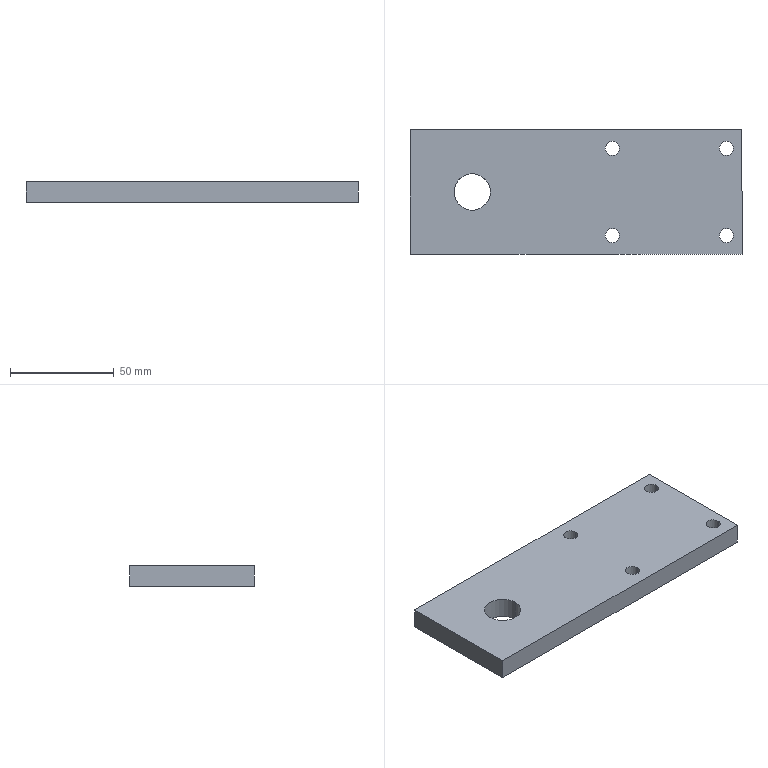Part | SolidWorks | features HoleWzd 2, Extrusion 1 | 1 solid | 16 faces | box 160 x 60 x 10 mm | volume 92142 mm3 | cylinder 10 | plane 6 | commonest cylinder face diameters 6.8 x8 17.5 x2
STEP:
#1=CARTESIAN_POINT('',(14.1,21.,0.));
#2=VERTEX_POINT('',#1);
#3=CARTESIAN_POINT('',(20.9,21.,0.));
#4=VERTEX_POINT('',#3);
#5=CARTESIAN_POINT('',(17.5,21.,0.));
#6=DIRECTION('',(0.,0.,1.));
#7=DIRECTION('',(1.,0.,0.));
#8=AXIS2_PLACEMENT_3D('',#5,#6,#7);
#9=CIRCLE('',#8,3.4);
#10=EDGE_CURVE('',#2,#4,#9,.T.);
#11=ORIENTED_EDGE('',*,*,#10,.F.);
#12=CARTESIAN_POINT('',(14.1,21.,10.));
#13=VERTEX_POINT('',#12);
#14=CARTESIAN_POINT('',(14.1,21.,10.));
#15=DIRECTION('',(0.,0.,1.));
#16=VECTOR('',#15,1000.);
#17=LINE('',#14,#16);
#18=EDGE_CURVE('',#2,#13,#17,.T.);
#19=ORIENTED_EDGE('',*,*,#18,.T.);
#20=CARTESIAN_POINT('',(20.9,21.,10.));
#21=VERTEX_POINT('',#20);
#22=CARTESIAN_POINT('',(17.5,21.,10.));
#23=DIRECTION('',(0.,0.,1.));
#24=DIRECTION('',(1.,0.,0.));
#25=AXIS2_PLACEMENT_3D('',#22,#23,#24);
#26=CIRCLE('',#25,3.4);
#27=EDGE_CURVE('',#13,#21,#26,.T.);
#28=ORIENTED_EDGE('',*,*,#27,.T.);
#29=CARTESIAN_POINT('',(20.9,21.,10.));
#30=DIRECTION('',(0.,0.,1.));
#31=VECTOR('',#30,1000.);
#32=LINE('',#29,#31);
#33=EDGE_CURVE('',#4,#21,#32,.T.);
#34=ORIENTED_EDGE('',*,*,#33,.F.);
#35=EDGE_LOOP('',(#11,#19,#28,#34));
#36=FACE_OUTER_BOUND('',#35,.T.);
#37=CARTESIAN_POINT('',(17.5,21.,10.));
#38=DIRECTION('',(0.,0.,1.));
#39=DIRECTION('',(1.,0.,0.));
#40=AXIS2_PLACEMENT_3D('',#37,#38,#39);
#41=CYLINDRICAL_SURFACE('',#40,3.4);
#42=ADVANCED_FACE('',(#36),#41,.F.);
#43=CARTESIAN_POINT('',(69.1,21.,0.));
#44=VERTEX_POINT('',#43);
#45=CARTESIAN_POINT('',(75.9,21.,0.));
#46=VERTEX_POINT('',#45);
#47=CARTESIAN_POINT('',(72.5,21.,0.));
#48=DIRECTION('',(0.,0.,1.));
#49=DIRECTION('',(1.,0.,0.));
#50=AXIS2_PLACEMENT_3D('',#47,#48,#49);
#51=CIRCLE('',#50,3.4);
#52=EDGE_CURVE('',#44,#46,#51,.T.);
#53=ORIENTED_EDGE('',*,*,#52,.F.);
#54=CARTESIAN_POINT('',(69.1,21.,10.));
#55=VERTEX_POINT('',#54);
#56=CARTESIAN_POINT('',(69.1,21.,10.));
#57=DIRECTION('',(0.,0.,1.));
#58=VECTOR('',#57,1000.);
#59=LINE('',#56,#58);
#60=EDGE_CURVE('',#44,#55,#59,.T.);
#61=ORIENTED_EDGE('',*,*,#60,.T.);
#62=CARTESIAN_POINT('',(75.9,21.,10.));
#63=VERTEX_POINT('',#62);
#64=CARTESIAN_POINT('',(72.5,21.,10.));
#65=DIRECTION('',(0.,0.,1.));
#66=DIRECTION('',(1.,0.,0.));
#67=AXIS2_PLACEMENT_3D('',#64,#65,#66);
#68=CIRCLE('',#67,3.4);
#69=EDGE_CURVE('',#55,#63,#68,.T.);
#70=ORIENTED_EDGE('',*,*,#69,.T.);
#71=CARTESIAN_POINT('',(75.9,21.,10.));
#72=DIRECTION('',(0.,0.,1.));
#73=VECTOR('',#72,1000.);
#74=LINE('',#71,#73);
#75=EDGE_CURVE('',#46,#63,#74,.T.);
#76=ORIENTED_EDGE('',*,*,#75,.F.);
#77=EDGE_LOOP('',(#53,#61,#70,#76));
#78=FACE_OUTER_BOUND('',#77,.T.);
#79=CARTESIAN_POINT('',(72.5,21.,10.));
#80=DIRECTION('',(0.,0.,1.));
#81=DIRECTION('',(1.,0.,0.));
#82=AXIS2_PLACEMENT_3D('',#79,#80,#81);
#83=CYLINDRICAL_SURFACE('',#82,3.4);
#84=ADVANCED_FACE('',(#78),#83,.F.);
#85=CARTESIAN_POINT('',(14.1,-21.,0.));
#86=VERTEX_POINT('',#85);
#87=CARTESIAN_POINT('',(20.9,-21.,0.));
#88=VERTEX_POINT('',#87);
#89=CARTESIAN_POINT('',(17.5,-21.,0.));
#90=DIRECTION('',(0.,0.,1.));
#91=DIRECTION('',(1.,0.,0.));
#92=AXIS2_PLACEMENT_3D('',#89,#90,#91);
#93=CIRCLE('',#92,3.4);
#94=EDGE_CURVE('',#86,#88,#93,.T.);
#95=ORIENTED_EDGE('',*,*,#94,.F.);
#96=CARTESIAN_POINT('',(14.1,-21.,10.));
#97=VERTEX_POINT('',#96);
#98=CARTESIAN_POINT('',(14.1,-21.,10.));
#99=DIRECTION('',(0.,0.,1.));
#100=VECTOR('',#99,1000.);
#101=LINE('',#98,#100);
#102=EDGE_CURVE('',#86,#97,#101,.T.);
#103=ORIENTED_EDGE('',*,*,#102,.T.);
#104=CARTESIAN_POINT('',(20.9,-21.,10.));
#105=VERTEX_POINT('',#104);
#106=CARTESIAN_POINT('',(17.5,-21.,10.));
#107=DIRECTION('',(0.,0.,1.));
#108=DIRECTION('',(1.,0.,0.));
#109=AXIS2_PLACEMENT_3D('',#106,#107,#108);
#110=CIRCLE('',#109,3.4);
#111=EDGE_CURVE('',#97,#105,#110,.T.);
#112=ORIENTED_EDGE('',*,*,#111,.T.);
#113=CARTESIAN_POINT('',(20.9,-21.,10.));
#114=DIRECTION('',(0.,0.,1.));
#115=VECTOR('',#114,1000.);
#116=LINE('',#113,#115);
#117=EDGE_CURVE('',#88,#105,#116,.T.);
#118=ORIENTED_EDGE('',*,*,#117,.F.);
#119=EDGE_LOOP('',(#95,#103,#112,#118));
#120=FACE_OUTER_BOUND('',#119,.T.);
#121=CARTESIAN_POINT('',(17.5,-21.,10.));
#122=DIRECTION('',(0.,0.,1.));
#123=DIRECTION('',(1.,0.,0.));
#124=AXIS2_PLACEMENT_3D('',#121,#122,#123);
#125=CYLINDRICAL_SURFACE('',#124,3.4);
#126=ADVANCED_FACE('',(#120),#125,.F.);
#127=CARTESIAN_POINT('',(69.1,-21.,0.));
#128=VERTEX_POINT('',#127);
#129=CARTESIAN_POINT('',(75.9,-21.,0.));
#130=VERTEX_POINT('',#129);
#131=CARTESIAN_POINT('',(72.5,-21.,0.));
#132=DIRECTION('',(0.,0.,1.));
#133=DIRECTION('',(1.,0.,0.));
#134=AXIS2_PLACEMENT_3D('',#131,#132,#133);
#135=CIRCLE('',#134,3.4);
#136=EDGE_CURVE('',#128,#130,#135,.T.);
#137=ORIENTED_EDGE('',*,*,#136,.F.);
#138=CARTESIAN_POINT('',(69.1,-21.,10.));
#139=VERTEX_POINT('',#138);
#140=CARTESIAN_POINT('',(69.1,-21.,10.));
#141=DIRECTION('',(0.,0.,1.));
#142=VECTOR('',#141,1000.);
#143=LINE('',#140,#142);
#144=EDGE_CURVE('',#128,#139,#143,.T.);
#145=ORIENTED_EDGE('',*,*,#144,.T.);
#146=CARTESIAN_POINT('',(75.9,-21.,10.));
#147=VERTEX_POINT('',#146);
#148=CARTESIAN_POINT('',(72.5,-21.,10.));
#149=DIRECTION('',(0.,0.,1.));
#150=DIRECTION('',(1.,0.,0.));
#151=AXIS2_PLACEMENT_3D('',#148,#149,#150);
#152=CIRCLE('',#151,3.4);
#153=EDGE_CURVE('',#139,#147,#152,.T.);
#154=ORIENTED_EDGE('',*,*,#153,.T.);
#155=CARTESIAN_POINT('',(75.9,-21.,10.));
#156=DIRECTION('',(0.,0.,1.));
#157=VECTOR('',#156,1000.);
#158=LINE('',#155,#157);
#159=EDGE_CURVE('',#130,#147,#158,.T.);
#160=ORIENTED_EDGE('',*,*,#159,.F.);
#161=EDGE_LOOP('',(#137,#145,#154,#160));
#162=FACE_OUTER_BOUND('',#161,.T.);
#163=CARTESIAN_POINT('',(72.5,-21.,10.));
#164=DIRECTION('',(0.,0.,1.));
#165=DIRECTION('',(1.,0.,0.));
#166=AXIS2_PLACEMENT_3D('',#163,#164,#165);
#167=CYLINDRICAL_SURFACE('',#166,3.4);
#168=ADVANCED_FACE('',(#162),#167,.F.);
#169=CARTESIAN_POINT('',(-58.75,0.,0.));
#170=VERTEX_POINT('',#169);
#171=CARTESIAN_POINT('',(-41.25,0.,0.));
#172=VERTEX_POINT('',#171);
#173=CARTESIAN_POINT('',(-50.,0.,0.));
#174=DIRECTION('',(0.,0.,1.));
#175=DIRECTION('',(1.,0.,0.));
#176=AXIS2_PLACEMENT_3D('',#173,#174,#175);
#177=CIRCLE('',#176,8.75);
#178=EDGE_CURVE('',#170,#172,#177,.T.);
#179=ORIENTED_EDGE('',*,*,#178,.F.);
#180=CARTESIAN_POINT('',(-58.75,0.,10.));
#181=VERTEX_POINT('',#180);
#182=CARTESIAN_POINT('',(-58.75,0.,10.));
#183=DIRECTION('',(0.,0.,1.));
#184=VECTOR('',#183,1000.);
#185=LINE('',#182,#184);
#186=EDGE_CURVE('',#170,#181,#185,.T.);
#187=ORIENTED_EDGE('',*,*,#186,.T.);
#188=CARTESIAN_POINT('',(-41.25,0.,10.));
#189=VERTEX_POINT('',#188);
#190=CARTESIAN_POINT('',(-50.,0.,10.));
#191=DIRECTION('',(0.,0.,1.));
#192=DIRECTION('',(1.,0.,0.));
#193=AXIS2_PLACEMENT_3D('',#190,#191,#192);
#194=CIRCLE('',#193,8.75);
#195=EDGE_CURVE('',#181,#189,#194,.T.);
#196=ORIENTED_EDGE('',*,*,#195,.T.);
#197=CARTESIAN_POINT('',(-41.25,0.,10.));
#198=DIRECTION('',(0.,0.,1.));
#199=VECTOR('',#198,1000.);
#200=LINE('',#197,#199);
#201=EDGE_CURVE('',#172,#189,#200,.T.);
#202=ORIENTED_EDGE('',*,*,#201,.F.);
#203=EDGE_LOOP('',(#179,#187,#196,#202));
#204=FACE_OUTER_BOUND('',#203,.T.);
#205=CARTESIAN_POINT('',(-50.,0.,10.));
#206=DIRECTION('',(0.,0.,1.));
#207=DIRECTION('',(1.,0.,0.));
#208=AXIS2_PLACEMENT_3D('',#205,#206,#207);
#209=CYLINDRICAL_SURFACE('',#208,8.75);
#210=ADVANCED_FACE('',(#204),#209,.F.);
#211=CARTESIAN_POINT('',(80.,-30.,0.));
#212=VERTEX_POINT('',#211);
#213=CARTESIAN_POINT('',(80.,30.,0.));
#214=VERTEX_POINT('',#213);
#215=CARTESIAN_POINT('',(80.,30.,0.));
#216=DIRECTION('',(0.,1.,0.));
#217=VECTOR('',#216,1000.);
#218=LINE('',#215,#217);
#219=EDGE_CURVE('',#212,#214,#218,.T.);
#220=ORIENTED_EDGE('',*,*,#219,.T.);
#221=CARTESIAN_POINT('',(80.,30.,10.));
#222=VERTEX_POINT('',#221);
#223=CARTESIAN_POINT('',(80.,30.,10.));
#224=DIRECTION('',(0.,0.,-1.));
#225=VECTOR('',#224,1000.);
#226=LINE('',#223,#225);
#227=EDGE_CURVE('',#222,#214,#226,.T.);
#228=ORIENTED_EDGE('',*,*,#227,.F.);
#229=CARTESIAN_POINT('',(80.,-30.,10.));
#230=VERTEX_POINT('',#229);
#231=CARTESIAN_POINT('',(80.,30.,10.));
#232=DIRECTION('',(0.,1.,0.));
#233=VECTOR('',#232,1000.);
#234=LINE('',#231,#233);
#235=EDGE_CURVE('',#230,#222,#234,.T.);
#236=ORIENTED_EDGE('',*,*,#235,.F.);
#237=CARTESIAN_POINT('',(80.,-30.,10.));
#238=DIRECTION('',(0.,0.,-1.));
#239=VECTOR('',#238,1000.);
#240=LINE('',#237,#239);
#241=EDGE_CURVE('',#230,#212,#240,.T.);
#242=ORIENTED_EDGE('',*,*,#241,.T.);
#243=EDGE_LOOP('',(#220,#228,#236,#242));
#244=FACE_OUTER_BOUND('',#243,.T.);
#245=CARTESIAN_POINT('',(80.,30.,10.));
#246=DIRECTION('',(-1.,0.,0.));
#247=DIRECTION('',(0.,-1.,0.));
#248=AXIS2_PLACEMENT_3D('',#245,#246,#247);
#249=PLANE('',#248);
#250=ADVANCED_FACE('',(#244),#249,.F.);
#251=CARTESIAN_POINT('',(-80.,30.,0.));
#252=VERTEX_POINT('',#251);
#253=CARTESIAN_POINT('',(-80.,30.,0.));
#254=DIRECTION('',(-1.,0.,0.));
#255=VECTOR('',#254,1000.);
#256=LINE('',#253,#255);
#257=EDGE_CURVE('',#214,#252,#256,.T.);
#258=ORIENTED_EDGE('',*,*,#257,.T.);
#259=CARTESIAN_POINT('',(-80.,30.,10.));
#260=VERTEX_POINT('',#259);
#261=CARTESIAN_POINT('',(-80.,30.,10.));
#262=DIRECTION('',(0.,0.,-1.));
#263=VECTOR('',#262,1000.);
#264=LINE('',#261,#263);
#265=EDGE_CURVE('',#260,#252,#264,.T.);
#266=ORIENTED_EDGE('',*,*,#265,.F.);
#267=CARTESIAN_POINT('',(-80.,30.,10.));
#268=DIRECTION('',(-1.,0.,0.));
#269=VECTOR('',#268,1000.);
#270=LINE('',#267,#269);
#271=EDGE_CURVE('',#222,#260,#270,.T.);
#272=ORIENTED_EDGE('',*,*,#271,.F.);
#273=ORIENTED_EDGE('',*,*,#227,.T.);
#274=EDGE_LOOP('',(#258,#266,#272,#273));
#275=FACE_OUTER_BOUND('',#274,.T.);
#276=CARTESIAN_POINT('',(-80.,30.,10.));
#277=DIRECTION('',(0.,-1.,0.));
#278=DIRECTION('',(0.,0.,-1.));
#279=AXIS2_PLACEMENT_3D('',#276,#277,#278);
#280=PLANE('',#279);
#281=ADVANCED_FACE('',(#275),#280,.F.);
#282=CARTESIAN_POINT('',(-80.,-30.,0.));
#283=VERTEX_POINT('',#282);
#284=CARTESIAN_POINT('',(-80.,30.,0.));
#285=DIRECTION('',(0.,-1.,0.));
#286=VECTOR('',#285,1000.);
#287=LINE('',#284,#286);
#288=EDGE_CURVE('',#252,#283,#287,.T.);
#289=ORIENTED_EDGE('',*,*,#288,.T.);
#290=CARTESIAN_POINT('',(-80.,-30.,10.));
#291=VERTEX_POINT('',#290);
#292=CARTESIAN_POINT('',(-80.,-30.,10.));
#293=DIRECTION('',(0.,0.,-1.));
#294=VECTOR('',#293,1000.);
#295=LINE('',#292,#294);
#296=EDGE_CURVE('',#291,#283,#295,.T.);
#297=ORIENTED_EDGE('',*,*,#296,.F.);
#298=CARTESIAN_POINT('',(-80.,30.,10.));
#299=DIRECTION('',(0.,-1.,0.));
#300=VECTOR('',#299,1000.);
#301=LINE('',#298,#300);
#302=EDGE_CURVE('',#260,#291,#301,.T.);
#303=ORIENTED_EDGE('',*,*,#302,.F.);
#304=ORIENTED_EDGE('',*,*,#265,.T.);
#305=EDGE_LOOP('',(#289,#297,#303,#304));
#306=FACE_OUTER_BOUND('',#305,.T.);
#307=CARTESIAN_POINT('',(-80.,30.,10.));
#308=DIRECTION('',(1.,0.,0.));
#309=DIRECTION('',(0.,1.,0.));
#310=AXIS2_PLACEMENT_3D('',#307,#308,#309);
#311=PLANE('',#310);
#312=ADVANCED_FACE('',(#306),#311,.F.);
#313=CARTESIAN_POINT('',(-80.,-30.,0.));
#314=DIRECTION('',(1.,0.,0.));
#315=VECTOR('',#314,1000.);
#316=LINE('',#313,#315);
#317=EDGE_CURVE('',#283,#212,#316,.T.);
#318=ORIENTED_EDGE('',*,*,#317,.T.);
#319=ORIENTED_EDGE('',*,*,#241,.F.);
#320=CARTESIAN_POINT('',(-80.,-30.,10.));
#321=DIRECTION('',(1.,0.,0.));
#322=VECTOR('',#321,1000.);
#323=LINE('',#320,#322);
#324=EDGE_CURVE('',#291,#230,#323,.T.);
#325=ORIENTED_EDGE('',*,*,#324,.F.);
#326=ORIENTED_EDGE('',*,*,#296,.T.);
#327=EDGE_LOOP('',(#318,#319,#325,#326));
#328=FACE_OUTER_BOUND('',#327,.T.);
#329=CARTESIAN_POINT('',(-80.,-30.,10.));
#330=DIRECTION('',(0.,1.,0.));
#331=DIRECTION('',(0.,0.,1.));
#332=AXIS2_PLACEMENT_3D('',#329,#330,#331);
#333=PLANE('',#332);
#334=ADVANCED_FACE('',(#328),#333,.F.);
#335=CARTESIAN_POINT('',(17.5,21.,10.));
#336=DIRECTION('',(0.,0.,1.));
#337=DIRECTION('',(1.,0.,0.));
#338=AXIS2_PLACEMENT_3D('',#335,#336,#337);
#339=CIRCLE('',#338,3.4);
#340=EDGE_CURVE('',#21,#13,#339,.T.);
#341=ORIENTED_EDGE('',*,*,#340,.F.);
#342=ORIENTED_EDGE('',*,*,#27,.F.);
#343=EDGE_LOOP('',(#341,#342));
#344=FACE_BOUND('',#343,.T.);
#345=CARTESIAN_POINT('',(72.5,21.,10.));
#346=DIRECTION('',(0.,0.,1.));
#347=DIRECTION('',(1.,0.,0.));
#348=AXIS2_PLACEMENT_3D('',#345,#346,#347);
#349=CIRCLE('',#348,3.4);
#350=EDGE_CURVE('',#63,#55,#349,.T.);
#351=ORIENTED_EDGE('',*,*,#350,.F.);
#352=ORIENTED_EDGE('',*,*,#69,.F.);
#353=EDGE_LOOP('',(#351,#352));
#354=FACE_BOUND('',#353,.T.);
#355=CARTESIAN_POINT('',(17.5,-21.,10.));
#356=DIRECTION('',(0.,0.,1.));
#357=DIRECTION('',(1.,0.,0.));
#358=AXIS2_PLACEMENT_3D('',#355,#356,#357);
#359=CIRCLE('',#358,3.4);
#360=EDGE_CURVE('',#105,#97,#359,.T.);
#361=ORIENTED_EDGE('',*,*,#360,.F.);
#362=ORIENTED_EDGE('',*,*,#111,.F.);
#363=EDGE_LOOP('',(#361,#362));
#364=FACE_BOUND('',#363,.T.);
#365=CARTESIAN_POINT('',(72.5,-21.,10.));
#366=DIRECTION('',(0.,0.,1.));
#367=DIRECTION('',(1.,0.,0.));
#368=AXIS2_PLACEMENT_3D('',#365,#366,#367);
#369=CIRCLE('',#368,3.4);
#370=EDGE_CURVE('',#147,#139,#369,.T.);
#371=ORIENTED_EDGE('',*,*,#370,.F.);
#372=ORIENTED_EDGE('',*,*,#153,.F.);
#373=EDGE_LOOP('',(#371,#372));
#374=FACE_BOUND('',#373,.T.);
#375=CARTESIAN_POINT('',(-50.,0.,10.));
#376=DIRECTION('',(0.,0.,1.));
#377=DIRECTION('',(1.,0.,0.));
#378=AXIS2_PLACEMENT_3D('',#375,#376,#377);
#379=CIRCLE('',#378,8.75);
#380=EDGE_CURVE('',#189,#181,#379,.T.);
#381=ORIENTED_EDGE('',*,*,#380,.F.);
#382=ORIENTED_EDGE('',*,*,#195,.F.);
#383=EDGE_LOOP('',(#381,#382));
#384=FACE_BOUND('',#383,.T.);
#385=ORIENTED_EDGE('',*,*,#235,.T.);
#386=ORIENTED_EDGE('',*,*,#271,.T.);
#387=ORIENTED_EDGE('',*,*,#302,.T.);
#388=ORIENTED_EDGE('',*,*,#324,.T.);
#389=EDGE_LOOP('',(#385,#386,#387,#388));
#390=FACE_OUTER_BOUND('',#389,.T.);
#391=CARTESIAN_POINT('',(0.,0.,10.));
#392=DIRECTION('',(0.,0.,1.));
#393=DIRECTION('',(1.,0.,0.));
#394=AXIS2_PLACEMENT_3D('',#391,#392,#393);
#395=PLANE('',#394);
#396=ADVANCED_FACE('',(#344,#354,#364,#374,#384,#390),#395,.T.);
#397=CARTESIAN_POINT('',(17.5,21.,0.));
#398=DIRECTION('',(0.,0.,1.));
#399=DIRECTION('',(1.,0.,0.));
#400=AXIS2_PLACEMENT_3D('',#397,#398,#399);
#401=CIRCLE('',#400,3.4);
#402=EDGE_CURVE('',#4,#2,#401,.T.);
#403=ORIENTED_EDGE('',*,*,#402,.T.);
#404=ORIENTED_EDGE('',*,*,#10,.T.);
#405=EDGE_LOOP('',(#403,#404));
#406=FACE_BOUND('',#405,.T.);
#407=CARTESIAN_POINT('',(72.5,21.,0.));
#408=DIRECTION('',(0.,0.,1.));
#409=DIRECTION('',(1.,0.,0.));
#410=AXIS2_PLACEMENT_3D('',#407,#408,#409);
#411=CIRCLE('',#410,3.4);
#412=EDGE_CURVE('',#46,#44,#411,.T.);
#413=ORIENTED_EDGE('',*,*,#412,.T.);
#414=ORIENTED_EDGE('',*,*,#52,.T.);
#415=EDGE_LOOP('',(#413,#414));
#416=FACE_BOUND('',#415,.T.);
#417=CARTESIAN_POINT('',(17.5,-21.,0.));
#418=DIRECTION('',(0.,0.,1.));
#419=DIRECTION('',(1.,0.,0.));
#420=AXIS2_PLACEMENT_3D('',#417,#418,#419);
#421=CIRCLE('',#420,3.4);
#422=EDGE_CURVE('',#88,#86,#421,.T.);
#423=ORIENTED_EDGE('',*,*,#422,.T.);
#424=ORIENTED_EDGE('',*,*,#94,.T.);
#425=EDGE_LOOP('',(#423,#424));
#426=FACE_BOUND('',#425,.T.);
#427=CARTESIAN_POINT('',(72.5,-21.,0.));
#428=DIRECTION('',(0.,0.,1.));
#429=DIRECTION('',(1.,0.,0.));
#430=AXIS2_PLACEMENT_3D('',#427,#428,#429);
#431=CIRCLE('',#430,3.4);
#432=EDGE_CURVE('',#130,#128,#431,.T.);
#433=ORIENTED_EDGE('',*,*,#432,.T.);
#434=ORIENTED_EDGE('',*,*,#136,.T.);
#435=EDGE_LOOP('',(#433,#434));
#436=FACE_BOUND('',#435,.T.);
#437=CARTESIAN_POINT('',(-50.,0.,0.));
#438=DIRECTION('',(0.,0.,1.));
#439=DIRECTION('',(1.,0.,0.));
#440=AXIS2_PLACEMENT_3D('',#437,#438,#439);
#441=CIRCLE('',#440,8.75);
#442=EDGE_CURVE('',#172,#170,#441,.T.);
#443=ORIENTED_EDGE('',*,*,#442,.T.);
#444=ORIENTED_EDGE('',*,*,#178,.T.);
#445=EDGE_LOOP('',(#443,#444));
#446=FACE_BOUND('',#445,.T.);
#447=ORIENTED_EDGE('',*,*,#219,.F.);
#448=ORIENTED_EDGE('',*,*,#317,.F.);
#449=ORIENTED_EDGE('',*,*,#288,.F.);
#450=ORIENTED_EDGE('',*,*,#257,.F.);
#451=EDGE_LOOP('',(#447,#448,#449,#450));
#452=FACE_OUTER_BOUND('',#451,.T.);
#453=CARTESIAN_POINT('',(0.,0.,0.));
#454=DIRECTION('',(0.,0.,1.));
#455=DIRECTION('',(1.,0.,0.));
#456=AXIS2_PLACEMENT_3D('',#453,#454,#455);
#457=PLANE('',#456);
#458=ADVANCED_FACE('',(#406,#416,#426,#436,#446,#452),#457,.F.);
#459=ORIENTED_EDGE('',*,*,#186,.F.);
#460=ORIENTED_EDGE('',*,*,#442,.F.);
#461=ORIENTED_EDGE('',*,*,#201,.T.);
#462=ORIENTED_EDGE('',*,*,#380,.T.);
#463=EDGE_LOOP('',(#459,#460,#461,#462));
#464=FACE_OUTER_BOUND('',#463,.T.);
#465=CARTESIAN_POINT('',(-50.,0.,10.));
#466=DIRECTION('',(0.,0.,1.));
#467=DIRECTION('',(1.,0.,0.));
#468=AXIS2_PLACEMENT_3D('',#465,#466,#467);
#469=CYLINDRICAL_SURFACE('',#468,8.75);
#470=ADVANCED_FACE('',(#464),#469,.F.);
#471=ORIENTED_EDGE('',*,*,#144,.F.);
#472=ORIENTED_EDGE('',*,*,#432,.F.);
#473=ORIENTED_EDGE('',*,*,#159,.T.);
#474=ORIENTED_EDGE('',*,*,#370,.T.);
#475=EDGE_LOOP('',(#471,#472,#473,#474));
#476=FACE_OUTER_BOUND('',#475,.T.);
#477=CARTESIAN_POINT('',(72.5,-21.,10.));
#478=DIRECTION('',(0.,0.,1.));
#479=DIRECTION('',(1.,0.,0.));
#480=AXIS2_PLACEMENT_3D('',#477,#478,#479);
#481=CYLINDRICAL_SURFACE('',#480,3.4);
#482=ADVANCED_FACE('',(#476),#481,.F.);
#483=ORIENTED_EDGE('',*,*,#102,.F.);
#484=ORIENTED_EDGE('',*,*,#422,.F.);
#485=ORIENTED_EDGE('',*,*,#117,.T.);
#486=ORIENTED_EDGE('',*,*,#360,.T.);
#487=EDGE_LOOP('',(#483,#484,#485,#486));
#488=FACE_OUTER_BOUND('',#487,.T.);
#489=CARTESIAN_POINT('',(17.5,-21.,10.));
#490=DIRECTION('',(0.,0.,1.));
#491=DIRECTION('',(1.,0.,0.));
#492=AXIS2_PLACEMENT_3D('',#489,#490,#491);
#493=CYLINDRICAL_SURFACE('',#492,3.4);
#494=ADVANCED_FACE('',(#488),#493,.F.);
#495=ORIENTED_EDGE('',*,*,#60,.F.);
#496=ORIENTED_EDGE('',*,*,#412,.F.);
#497=ORIENTED_EDGE('',*,*,#75,.T.);
#498=ORIENTED_EDGE('',*,*,#350,.T.);
#499=EDGE_LOOP('',(#495,#496,#497,#498));
#500=FACE_OUTER_BOUND('',#499,.T.);
#501=CARTESIAN_POINT('',(72.5,21.,10.));
#502=DIRECTION('',(0.,0.,1.));
#503=DIRECTION('',(1.,0.,0.));
#504=AXIS2_PLACEMENT_3D('',#501,#502,#503);
#505=CYLINDRICAL_SURFACE('',#504,3.4);
#506=ADVANCED_FACE('',(#500),#505,.F.);
#507=ORIENTED_EDGE('',*,*,#18,.F.);
#508=ORIENTED_EDGE('',*,*,#402,.F.);
#509=ORIENTED_EDGE('',*,*,#33,.T.);
#510=ORIENTED_EDGE('',*,*,#340,.T.);
#511=EDGE_LOOP('',(#507,#508,#509,#510));
#512=FACE_OUTER_BOUND('',#511,.T.);
#513=CARTESIAN_POINT('',(17.5,21.,10.));
#514=DIRECTION('',(0.,0.,1.));
#515=DIRECTION('',(1.,0.,0.));
#516=AXIS2_PLACEMENT_3D('',#513,#514,#515);
#517=CYLINDRICAL_SURFACE('',#516,3.4);
#518=ADVANCED_FACE('',(#512),#517,.F.);
#519=CLOSED_SHELL('',(#42,#84,#126,#168,#210,#250,#281,#312,#334,#396,#458,#470,#482,#494,#506,#518));
#520=MANIFOLD_SOLID_BREP('',#519);
#521=CARTESIAN_POINT('',(0.,0.,0.));
#522=DIRECTION('',(0.,0.,1.));
#523=DIRECTION('',(1.,0.,0.));
#524=AXIS2_PLACEMENT_3D('',#521,#522,#523);
#525=(LENGTH_UNIT()NAMED_UNIT(*)SI_UNIT(.MILLI.,.METRE.));
#526=UNCERTAINTY_MEASURE_WITH_UNIT(LENGTH_MEASURE(0.00001),#525,'','');
#527=(NAMED_UNIT(*)PLANE_ANGLE_UNIT()SI_UNIT($,.RADIAN.));
#528=(NAMED_UNIT(*)SI_UNIT($,.STERADIAN.)SOLID_ANGLE_UNIT());
#529=(GEOMETRIC_REPRESENTATION_CONTEXT(3)GLOBAL_UNCERTAINTY_ASSIGNED_CONTEXT((#526))GLOBAL_UNIT_ASSIGNED_CONTEXT((#525,#527,#528))REPRESENTATION_CONTEXT('',''));
#530=ADVANCED_BREP_SHAPE_REPRESENTATION('',(#520,#524),#529);